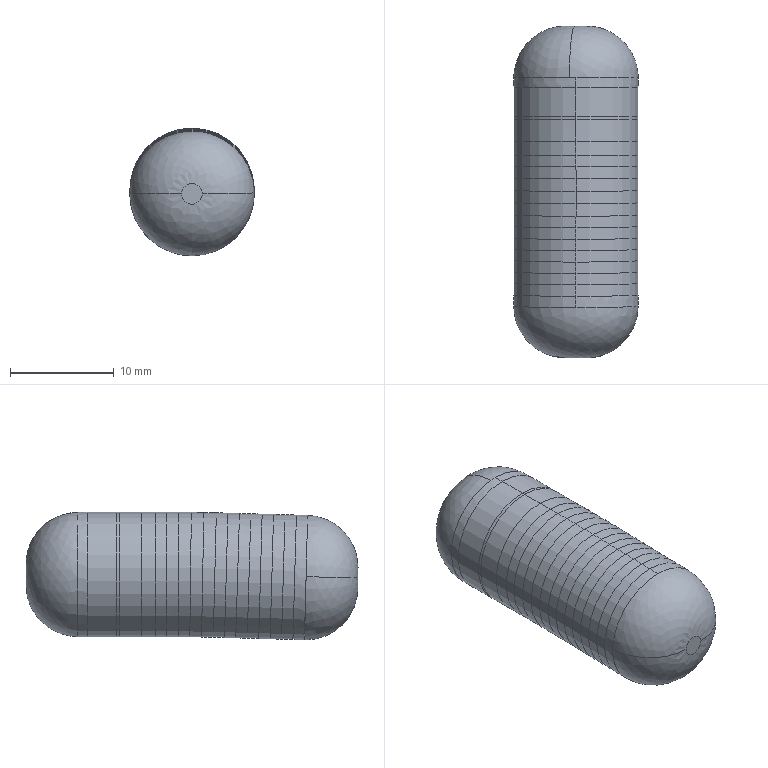Part | Creo | 1 solid | 43 faces | box 12 x 32.007 x 12.304 mm | volume 3289 mm3 | torus 37 | spline 4 | plane 2